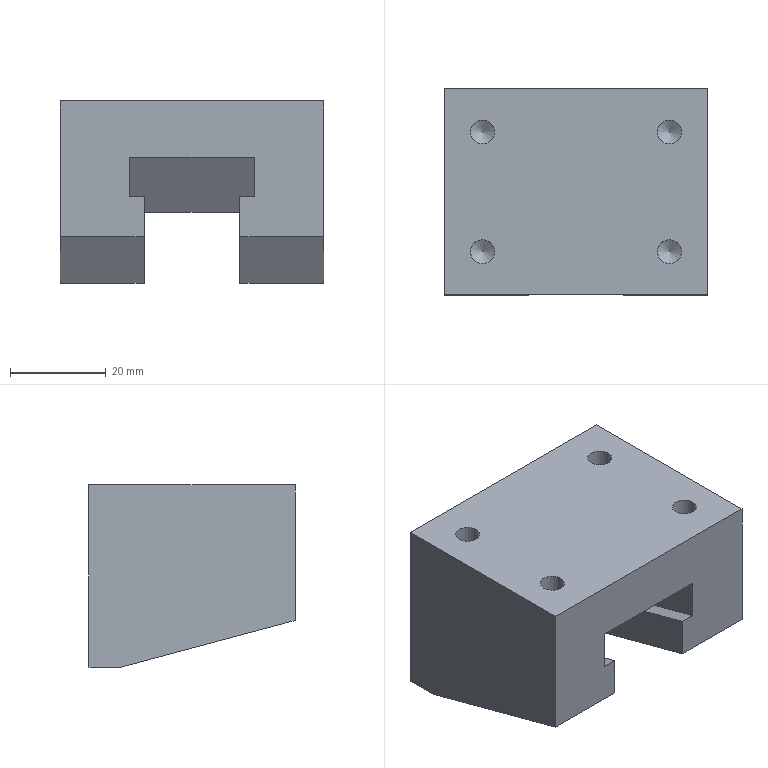Part | STEP file | lll_id478_x_t | 1 solid | 24 faces | box 55 x 43 x 38 mm | volume 62976 mm3 | plane 16 | cone 4 | cylinder 4 | commonest cylinder face diameters 5 x4
STEP:
#1=CARTESIAN_POINT('',(-27.5,108.,137.5));
#2=VERTEX_POINT('',#1);
#3=CARTESIAN_POINT('',(-27.5,108.,99.5));
#4=VERTEX_POINT('',#3);
#5=CARTESIAN_POINT('',(-27.5,108.,83.875));
#6=DIRECTION('',(0.,0.,-1.));
#7=VECTOR('',#6,1.);
#8=LINE('',#5,#7);
#9=EDGE_CURVE('',#2,#4,#8,.T.);
#10=ORIENTED_EDGE('',*,*,#9,.T.);
#11=CARTESIAN_POINT('',(-27.5,101.196,99.5));
#12=VERTEX_POINT('',#11);
#13=CARTESIAN_POINT('',(-27.5,140.161,99.5));
#14=DIRECTION('',(0.,-1.,0.));
#15=VECTOR('',#14,1.);
#16=LINE('',#13,#15);
#17=EDGE_CURVE('',#4,#12,#16,.T.);
#18=ORIENTED_EDGE('',*,*,#17,.T.);
#19=CARTESIAN_POINT('',(-27.5,65.,109.199));
#20=VERTEX_POINT('',#19);
#21=CARTESIAN_POINT('',(-27.5,141.457,88.712));
#22=DIRECTION('',(0.,0.9659,-0.2588));
#23=VECTOR('',#22,1.);
#24=LINE('',#21,#23);
#25=EDGE_CURVE('',#20,#12,#24,.T.);
#26=ORIENTED_EDGE('',*,*,#25,.F.);
#27=CARTESIAN_POINT('',(-27.5,65.,137.5));
#28=VERTEX_POINT('',#27);
#29=CARTESIAN_POINT('',(-27.5,65.,30.5));
#30=DIRECTION('',(0.,0.,-1.));
#31=VECTOR('',#30,1.);
#32=LINE('',#29,#31);
#33=EDGE_CURVE('',#28,#20,#32,.T.);
#34=ORIENTED_EDGE('',*,*,#33,.F.);
#35=CARTESIAN_POINT('',(-27.5,0.,137.5));
#36=DIRECTION('',(0.,-1.,0.));
#37=VECTOR('',#36,1.);
#38=LINE('',#35,#37);
#39=EDGE_CURVE('',#2,#28,#38,.T.);
#40=ORIENTED_EDGE('',*,*,#39,.F.);
#41=EDGE_LOOP('',(#10,#18,#26,#34,#40));
#42=FACE_OUTER_BOUND('',#41,.T.);
#43=CARTESIAN_POINT('',(-27.5,140.161,83.875));
#44=DIRECTION('',(-1.,0.,0.));
#45=DIRECTION('',(0.,0.,1.));
#46=AXIS2_PLACEMENT_3D('',#43,#44,#45);
#47=PLANE('',#46);
#48=ADVANCED_FACE('',(#42),#47,.T.);
#49=CARTESIAN_POINT('',(27.5,101.196,99.5));
#50=VERTEX_POINT('',#49);
#51=CARTESIAN_POINT('',(27.5,65.,109.199));
#52=VERTEX_POINT('',#51);
#53=CARTESIAN_POINT('',(27.5,141.457,88.712));
#54=DIRECTION('',(0.,-0.9659,0.2588));
#55=VECTOR('',#54,1.);
#56=LINE('',#53,#55);
#57=EDGE_CURVE('',#50,#52,#56,.T.);
#58=ORIENTED_EDGE('',*,*,#57,.F.);
#59=CARTESIAN_POINT('',(27.5,108.,99.5));
#60=VERTEX_POINT('',#59);
#61=CARTESIAN_POINT('',(27.5,140.161,99.5));
#62=DIRECTION('',(0.,1.,0.));
#63=VECTOR('',#62,1.);
#64=LINE('',#61,#63);
#65=EDGE_CURVE('',#50,#60,#64,.T.);
#66=ORIENTED_EDGE('',*,*,#65,.T.);
#67=CARTESIAN_POINT('',(27.5,108.,137.5));
#68=VERTEX_POINT('',#67);
#69=CARTESIAN_POINT('',(27.5,108.,83.875));
#70=DIRECTION('',(0.,0.,1.));
#71=VECTOR('',#70,1.);
#72=LINE('',#69,#71);
#73=EDGE_CURVE('',#60,#68,#72,.T.);
#74=ORIENTED_EDGE('',*,*,#73,.T.);
#75=CARTESIAN_POINT('',(27.5,65.,137.5));
#76=VERTEX_POINT('',#75);
#77=CARTESIAN_POINT('',(27.5,140.161,137.5));
#78=DIRECTION('',(0.,-1.,0.));
#79=VECTOR('',#78,1.);
#80=LINE('',#77,#79);
#81=EDGE_CURVE('',#68,#76,#80,.T.);
#82=ORIENTED_EDGE('',*,*,#81,.T.);
#83=CARTESIAN_POINT('',(27.5,65.,83.875));
#84=DIRECTION('',(0.,0.,-1.));
#85=VECTOR('',#84,1.);
#86=LINE('',#83,#85);
#87=EDGE_CURVE('',#76,#52,#86,.T.);
#88=ORIENTED_EDGE('',*,*,#87,.T.);
#89=EDGE_LOOP('',(#58,#66,#74,#82,#88));
#90=FACE_OUTER_BOUND('',#89,.T.);
#91=CARTESIAN_POINT('',(27.5,140.161,83.875));
#92=DIRECTION('',(1.,0.,0.));
#93=DIRECTION('',(0.,0.,-1.));
#94=AXIS2_PLACEMENT_3D('',#91,#92,#93);
#95=PLANE('',#94);
#96=ADVANCED_FACE('',(#90),#95,.T.);
#97=ORIENTED_EDGE('',*,*,#73,.F.);
#98=CARTESIAN_POINT('',(10.,108.,99.5));
#99=VERTEX_POINT('',#98);
#100=CARTESIAN_POINT('',(0.,108.,99.5));
#101=DIRECTION('',(-1.,0.,0.));
#102=VECTOR('',#101,1.);
#103=LINE('',#100,#102);
#104=EDGE_CURVE('',#60,#99,#103,.T.);
#105=ORIENTED_EDGE('',*,*,#104,.T.);
#106=CARTESIAN_POINT('',(10.,108.,105.959));
#107=VERTEX_POINT('',#106);
#108=CARTESIAN_POINT('',(10.,108.,30.5));
#109=DIRECTION('',(0.,0.,-1.));
#110=VECTOR('',#109,1.);
#111=LINE('',#108,#110);
#112=EDGE_CURVE('',#107,#99,#111,.T.);
#113=ORIENTED_EDGE('',*,*,#112,.F.);
#114=CARTESIAN_POINT('',(13.,108.,105.959));
#115=VERTEX_POINT('',#114);
#116=CARTESIAN_POINT('',(0.,108.,105.959));
#117=DIRECTION('',(-1.,0.,0.));
#118=VECTOR('',#117,1.);
#119=LINE('',#116,#118);
#120=EDGE_CURVE('',#115,#107,#119,.T.);
#121=ORIENTED_EDGE('',*,*,#120,.F.);
#122=CARTESIAN_POINT('',(13.,108.,114.241));
#123=VERTEX_POINT('',#122);
#124=CARTESIAN_POINT('',(13.,108.,30.5));
#125=DIRECTION('',(0.,0.,-1.));
#126=VECTOR('',#125,1.);
#127=LINE('',#124,#126);
#128=EDGE_CURVE('',#123,#115,#127,.T.);
#129=ORIENTED_EDGE('',*,*,#128,.F.);
#130=CARTESIAN_POINT('',(-13.,108.,114.241));
#131=VERTEX_POINT('',#130);
#132=CARTESIAN_POINT('',(0.,108.,114.241));
#133=DIRECTION('',(-1.,0.,0.));
#134=VECTOR('',#133,1.);
#135=LINE('',#132,#134);
#136=EDGE_CURVE('',#123,#131,#135,.T.);
#137=ORIENTED_EDGE('',*,*,#136,.T.);
#138=CARTESIAN_POINT('',(-13.,108.,105.959));
#139=VERTEX_POINT('',#138);
#140=CARTESIAN_POINT('',(-13.,108.,30.5));
#141=DIRECTION('',(0.,0.,-1.));
#142=VECTOR('',#141,1.);
#143=LINE('',#140,#142);
#144=EDGE_CURVE('',#131,#139,#143,.T.);
#145=ORIENTED_EDGE('',*,*,#144,.T.);
#146=CARTESIAN_POINT('',(-10.,108.,105.959));
#147=VERTEX_POINT('',#146);
#148=CARTESIAN_POINT('',(0.,108.,105.959));
#149=DIRECTION('',(-1.,0.,0.));
#150=VECTOR('',#149,1.);
#151=LINE('',#148,#150);
#152=EDGE_CURVE('',#147,#139,#151,.T.);
#153=ORIENTED_EDGE('',*,*,#152,.F.);
#154=CARTESIAN_POINT('',(-10.,108.,99.5));
#155=VERTEX_POINT('',#154);
#156=CARTESIAN_POINT('',(-10.,108.,30.5));
#157=DIRECTION('',(0.,0.,-1.));
#158=VECTOR('',#157,1.);
#159=LINE('',#156,#158);
#160=EDGE_CURVE('',#147,#155,#159,.T.);
#161=ORIENTED_EDGE('',*,*,#160,.T.);
#162=CARTESIAN_POINT('',(0.,108.,99.5));
#163=DIRECTION('',(-1.,0.,0.));
#164=VECTOR('',#163,1.);
#165=LINE('',#162,#164);
#166=EDGE_CURVE('',#155,#4,#165,.T.);
#167=ORIENTED_EDGE('',*,*,#166,.T.);
#168=ORIENTED_EDGE('',*,*,#9,.F.);
#169=CARTESIAN_POINT('',(0.,108.,137.5));
#170=DIRECTION('',(-1.,0.,0.));
#171=VECTOR('',#170,1.);
#172=LINE('',#169,#171);
#173=EDGE_CURVE('',#68,#2,#172,.T.);
#174=ORIENTED_EDGE('',*,*,#173,.F.);
#175=EDGE_LOOP('',(#97,#105,#113,#121,#129,#137,#145,#153,#161,#167,#168,#174));
#176=FACE_OUTER_BOUND('',#175,.T.);
#177=CARTESIAN_POINT('',(0.,108.,30.5));
#178=DIRECTION('',(0.,1.,0.));
#179=DIRECTION('',(0.,0.,1.));
#180=AXIS2_PLACEMENT_3D('',#177,#178,#179);
#181=PLANE('',#180);
#182=ADVANCED_FACE('',(#176),#181,.T.);
#183=CARTESIAN_POINT('',(-10.,101.196,99.5));
#184=VERTEX_POINT('',#183);
#185=CARTESIAN_POINT('',(0.00001281,101.196,99.5));
#186=DIRECTION('',(-1.,0.,0.));
#187=VECTOR('',#186,1.);
#188=LINE('',#185,#187);
#189=EDGE_CURVE('',#184,#12,#188,.T.);
#190=ORIENTED_EDGE('',*,*,#189,.F.);
#191=CARTESIAN_POINT('',(-10.,65.,109.199));
#192=VERTEX_POINT('',#191);
#193=CARTESIAN_POINT('',(-10.,90.,102.5));
#194=DIRECTION('',(0.,0.9659,-0.2588));
#195=VECTOR('',#194,1.);
#196=LINE('',#193,#195);
#197=EDGE_CURVE('',#192,#184,#196,.T.);
#198=ORIENTED_EDGE('',*,*,#197,.F.);
#199=CARTESIAN_POINT('',(0.,65.,109.199));
#200=DIRECTION('',(-1.,0.,0.));
#201=VECTOR('',#200,1.);
#202=LINE('',#199,#201);
#203=EDGE_CURVE('',#192,#20,#202,.T.);
#204=ORIENTED_EDGE('',*,*,#203,.T.);
#205=ORIENTED_EDGE('',*,*,#25,.T.);
#206=EDGE_LOOP('',(#190,#198,#204,#205));
#207=FACE_OUTER_BOUND('',#206,.T.);
#208=CARTESIAN_POINT('',(0.00001281,90.,102.5));
#209=DIRECTION('',(0.,-0.2588,-0.9659));
#210=DIRECTION('',(0.,0.9659,-0.2588));
#211=AXIS2_PLACEMENT_3D('',#208,#209,#210);
#212=PLANE('',#211);
#213=ADVANCED_FACE('',(#207),#212,.T.);
#214=ORIENTED_EDGE('',*,*,#197,.T.);
#215=CARTESIAN_POINT('',(-10.,64.,99.5));
#216=DIRECTION('',(0.,1.,0.));
#217=VECTOR('',#216,1.);
#218=LINE('',#215,#217);
#219=EDGE_CURVE('',#184,#155,#218,.T.);
#220=ORIENTED_EDGE('',*,*,#219,.T.);
#221=ORIENTED_EDGE('',*,*,#160,.F.);
#222=CARTESIAN_POINT('',(-10.,65.,117.481));
#223=VERTEX_POINT('',#222);
#224=CARTESIAN_POINT('',(-10.,79.071,113.711));
#225=DIRECTION('',(0.,-0.9659,0.2588));
#226=VECTOR('',#225,1.);
#227=LINE('',#224,#226);
#228=EDGE_CURVE('',#147,#223,#227,.T.);
#229=ORIENTED_EDGE('',*,*,#228,.T.);
#230=CARTESIAN_POINT('',(-10.,65.,30.5));
#231=DIRECTION('',(0.,0.,1.));
#232=VECTOR('',#231,1.);
#233=LINE('',#230,#232);
#234=EDGE_CURVE('',#192,#223,#233,.T.);
#235=ORIENTED_EDGE('',*,*,#234,.F.);
#236=EDGE_LOOP('',(#214,#220,#221,#229,#235));
#237=FACE_OUTER_BOUND('',#236,.T.);
#238=CARTESIAN_POINT('',(-10.,64.,109.467));
#239=DIRECTION('',(1.,0.,0.));
#240=DIRECTION('',(0.,0.,-1.));
#241=AXIS2_PLACEMENT_3D('',#238,#239,#240);
#242=PLANE('',#241);
#243=ADVANCED_FACE('',(#237),#242,.T.);
#244=CARTESIAN_POINT('',(10.,101.196,99.5));
#245=VERTEX_POINT('',#244);
#246=CARTESIAN_POINT('',(0.00001281,101.196,99.5));
#247=DIRECTION('',(-1.,0.,0.));
#248=VECTOR('',#247,1.);
#249=LINE('',#246,#248);
#250=EDGE_CURVE('',#50,#245,#249,.T.);
#251=ORIENTED_EDGE('',*,*,#250,.F.);
#252=ORIENTED_EDGE('',*,*,#57,.T.);
#253=CARTESIAN_POINT('',(10.,65.,109.199));
#254=VERTEX_POINT('',#253);
#255=CARTESIAN_POINT('',(0.,65.,109.199));
#256=DIRECTION('',(-1.,0.,0.));
#257=VECTOR('',#256,1.);
#258=LINE('',#255,#257);
#259=EDGE_CURVE('',#52,#254,#258,.T.);
#260=ORIENTED_EDGE('',*,*,#259,.T.);
#261=CARTESIAN_POINT('',(10.,90.,102.5));
#262=DIRECTION('',(0.,0.9659,-0.2588));
#263=VECTOR('',#262,1.);
#264=LINE('',#261,#263);
#265=EDGE_CURVE('',#254,#245,#264,.T.);
#266=ORIENTED_EDGE('',*,*,#265,.T.);
#267=EDGE_LOOP('',(#251,#252,#260,#266));
#268=FACE_OUTER_BOUND('',#267,.T.);
#269=CARTESIAN_POINT('',(0.00001281,90.,102.5));
#270=DIRECTION('',(0.,-0.2588,-0.9659));
#271=DIRECTION('',(0.,0.9659,-0.2588));
#272=AXIS2_PLACEMENT_3D('',#269,#270,#271);
#273=PLANE('',#272);
#274=ADVANCED_FACE('',(#268),#273,.T.);
#275=CARTESIAN_POINT('',(10.,64.,99.5));
#276=DIRECTION('',(0.,1.,0.));
#277=VECTOR('',#276,1.);
#278=LINE('',#275,#277);
#279=EDGE_CURVE('',#245,#99,#278,.T.);
#280=ORIENTED_EDGE('',*,*,#279,.F.);
#281=ORIENTED_EDGE('',*,*,#265,.F.);
#282=CARTESIAN_POINT('',(10.,65.,117.481));
#283=VERTEX_POINT('',#282);
#284=CARTESIAN_POINT('',(10.,65.,30.5));
#285=DIRECTION('',(0.,0.,1.));
#286=VECTOR('',#285,1.);
#287=LINE('',#284,#286);
#288=EDGE_CURVE('',#254,#283,#287,.T.);
#289=ORIENTED_EDGE('',*,*,#288,.T.);
#290=CARTESIAN_POINT('',(10.,79.071,113.711));
#291=DIRECTION('',(0.,-0.9659,0.2588));
#292=VECTOR('',#291,1.);
#293=LINE('',#290,#292);
#294=EDGE_CURVE('',#107,#283,#293,.T.);
#295=ORIENTED_EDGE('',*,*,#294,.F.);
#296=ORIENTED_EDGE('',*,*,#112,.T.);
#297=EDGE_LOOP('',(#280,#281,#289,#295,#296));
#298=FACE_OUTER_BOUND('',#297,.T.);
#299=CARTESIAN_POINT('',(10.,64.,109.467));
#300=DIRECTION('',(1.,0.,0.));
#301=DIRECTION('',(0.,0.,-1.));
#302=AXIS2_PLACEMENT_3D('',#299,#300,#301);
#303=PLANE('',#302);
#304=ADVANCED_FACE('',(#298),#303,.F.);
#305=ORIENTED_EDGE('',*,*,#136,.F.);
#306=CARTESIAN_POINT('',(13.,65.,125.763));
#307=VERTEX_POINT('',#306);
#308=CARTESIAN_POINT('',(13.,81.141,121.438));
#309=DIRECTION('',(0.,-0.9659,0.2588));
#310=VECTOR('',#309,1.);
#311=LINE('',#308,#310);
#312=EDGE_CURVE('',#123,#307,#311,.T.);
#313=ORIENTED_EDGE('',*,*,#312,.T.);
#314=CARTESIAN_POINT('',(-13.,65.,125.763));
#315=VERTEX_POINT('',#314);
#316=CARTESIAN_POINT('',(0.,65.,125.763));
#317=DIRECTION('',(1.,0.,0.));
#318=VECTOR('',#317,1.);
#319=LINE('',#316,#318);
#320=EDGE_CURVE('',#315,#307,#319,.T.);
#321=ORIENTED_EDGE('',*,*,#320,.F.);
#322=CARTESIAN_POINT('',(-13.,81.141,121.438));
#323=DIRECTION('',(0.,-0.9659,0.2588));
#324=VECTOR('',#323,1.);
#325=LINE('',#322,#324);
#326=EDGE_CURVE('',#131,#315,#325,.T.);
#327=ORIENTED_EDGE('',*,*,#326,.F.);
#328=EDGE_LOOP('',(#305,#313,#321,#327));
#329=FACE_OUTER_BOUND('',#328,.T.);
#330=CARTESIAN_POINT('',(0.00001281,81.141,121.438));
#331=DIRECTION('',(0.,-0.2588,-0.9659));
#332=DIRECTION('',(0.,0.9659,-0.2588));
#333=AXIS2_PLACEMENT_3D('',#330,#331,#332);
#334=PLANE('',#333);
#335=ADVANCED_FACE('',(#329),#334,.T.);
#336=CARTESIAN_POINT('',(22.,99.,137.5));
#337=VERTEX_POINT('',#336);
#338=CARTESIAN_POINT('',(19.5,99.,137.5));
#339=DIRECTION('',(0.,0.,-1.));
#340=DIRECTION('',(1.,0.,0.));
#341=AXIS2_PLACEMENT_3D('',#338,#339,#340);
#342=CIRCLE('',#341,2.5);
#343=EDGE_CURVE('',#337,#337,#342,.T.);
#344=ORIENTED_EDGE('',*,*,#343,.T.);
#345=EDGE_LOOP('',(#344));
#346=FACE_BOUND('',#345,.T.);
#347=CARTESIAN_POINT('',(22.,74.,137.5));
#348=VERTEX_POINT('',#347);
#349=CARTESIAN_POINT('',(19.5,74.,137.5));
#350=DIRECTION('',(0.,0.,1.));
#351=DIRECTION('',(1.,0.,0.));
#352=AXIS2_PLACEMENT_3D('',#349,#350,#351);
#353=CIRCLE('',#352,2.5);
#354=EDGE_CURVE('',#348,#348,#353,.T.);
#355=ORIENTED_EDGE('',*,*,#354,.F.);
#356=EDGE_LOOP('',(#355));
#357=FACE_BOUND('',#356,.T.);
#358=CARTESIAN_POINT('',(-22.,99.,137.5));
#359=VERTEX_POINT('',#358);
#360=CARTESIAN_POINT('',(-19.5,99.,137.5));
#361=DIRECTION('',(0.,0.,1.));
#362=DIRECTION('',(-1.,0.,0.));
#363=AXIS2_PLACEMENT_3D('',#360,#361,#362);
#364=CIRCLE('',#363,2.5);
#365=EDGE_CURVE('',#359,#359,#364,.T.);
#366=ORIENTED_EDGE('',*,*,#365,.F.);
#367=EDGE_LOOP('',(#366));
#368=FACE_BOUND('',#367,.T.);
#369=CARTESIAN_POINT('',(-22.,74.,137.5));
#370=VERTEX_POINT('',#369);
#371=CARTESIAN_POINT('',(-19.5,74.,137.5));
#372=DIRECTION('',(0.,0.,-1.));
#373=DIRECTION('',(-1.,0.,0.));
#374=AXIS2_PLACEMENT_3D('',#371,#372,#373);
#375=CIRCLE('',#374,2.5);
#376=EDGE_CURVE('',#370,#370,#375,.T.);
#377=ORIENTED_EDGE('',*,*,#376,.T.);
#378=EDGE_LOOP('',(#377));
#379=FACE_BOUND('',#378,.T.);
#380=CARTESIAN_POINT('',(0.,65.,137.5));
#381=DIRECTION('',(-1.,0.,0.));
#382=VECTOR('',#381,1.);
#383=LINE('',#380,#382);
#384=EDGE_CURVE('',#76,#28,#383,.T.);
#385=ORIENTED_EDGE('',*,*,#384,.F.);
#386=ORIENTED_EDGE('',*,*,#81,.F.);
#387=ORIENTED_EDGE('',*,*,#173,.T.);
#388=ORIENTED_EDGE('',*,*,#39,.T.);
#389=EDGE_LOOP('',(#385,#386,#387,#388));
#390=FACE_BOUND('',#389,.T.);
#391=CARTESIAN_POINT('',(0.,0.,137.5));
#392=DIRECTION('',(0.,0.,1.));
#393=DIRECTION('',(1.,0.,0.));
#394=AXIS2_PLACEMENT_3D('',#391,#392,#393);
#395=PLANE('',#394);
#396=ADVANCED_FACE('',(#346,#357,#368,#379,#390),#395,.T.);
#397=ORIENTED_EDGE('',*,*,#33,.T.);
#398=ORIENTED_EDGE('',*,*,#203,.F.);
#399=ORIENTED_EDGE('',*,*,#234,.T.);
#400=CARTESIAN_POINT('',(-13.,65.,117.481));
#401=VERTEX_POINT('',#400);
#402=CARTESIAN_POINT('',(0.,65.,117.481));
#403=DIRECTION('',(1.,0.,0.));
#404=VECTOR('',#403,1.);
#405=LINE('',#402,#404);
#406=EDGE_CURVE('',#401,#223,#405,.T.);
#407=ORIENTED_EDGE('',*,*,#406,.F.);
#408=CARTESIAN_POINT('',(-13.,65.,30.5));
#409=DIRECTION('',(0.,0.,1.));
#410=VECTOR('',#409,1.);
#411=LINE('',#408,#410);
#412=EDGE_CURVE('',#401,#315,#411,.T.);
#413=ORIENTED_EDGE('',*,*,#412,.T.);
#414=ORIENTED_EDGE('',*,*,#320,.T.);
#415=CARTESIAN_POINT('',(13.,65.,117.481));
#416=VERTEX_POINT('',#415);
#417=CARTESIAN_POINT('',(13.,65.,30.5));
#418=DIRECTION('',(0.,0.,1.));
#419=VECTOR('',#418,1.);
#420=LINE('',#417,#419);
#421=EDGE_CURVE('',#416,#307,#420,.T.);
#422=ORIENTED_EDGE('',*,*,#421,.F.);
#423=CARTESIAN_POINT('',(0.,65.,117.481));
#424=DIRECTION('',(1.,0.,0.));
#425=VECTOR('',#424,1.);
#426=LINE('',#423,#425);
#427=EDGE_CURVE('',#283,#416,#426,.T.);
#428=ORIENTED_EDGE('',*,*,#427,.F.);
#429=ORIENTED_EDGE('',*,*,#288,.F.);
#430=ORIENTED_EDGE('',*,*,#259,.F.);
#431=ORIENTED_EDGE('',*,*,#87,.F.);
#432=ORIENTED_EDGE('',*,*,#384,.T.);
#433=EDGE_LOOP('',(#397,#398,#399,#407,#413,#414,#422,#428,#429,#430,#431,#432));
#434=FACE_OUTER_BOUND('',#433,.T.);
#435=CARTESIAN_POINT('',(0.,65.,30.5));
#436=DIRECTION('',(0.,1.,0.));
#437=DIRECTION('',(0.,0.,1.));
#438=AXIS2_PLACEMENT_3D('',#435,#436,#437);
#439=PLANE('',#438);
#440=ADVANCED_FACE('',(#434),#439,.F.);
#441=CARTESIAN_POINT('',(-13.,79.071,113.711));
#442=DIRECTION('',(0.,-0.9659,0.2588));
#443=VECTOR('',#442,1.);
#444=LINE('',#441,#443);
#445=EDGE_CURVE('',#139,#401,#444,.T.);
#446=ORIENTED_EDGE('',*,*,#445,.F.);
#447=ORIENTED_EDGE('',*,*,#144,.F.);
#448=ORIENTED_EDGE('',*,*,#326,.T.);
#449=ORIENTED_EDGE('',*,*,#412,.F.);
#450=EDGE_LOOP('',(#446,#447,#448,#449));
#451=FACE_OUTER_BOUND('',#450,.T.);
#452=CARTESIAN_POINT('',(-13.,64.,109.467));
#453=DIRECTION('',(1.,0.,0.));
#454=DIRECTION('',(0.,0.,-1.));
#455=AXIS2_PLACEMENT_3D('',#452,#453,#454);
#456=PLANE('',#455);
#457=ADVANCED_FACE('',(#451),#456,.T.);
#458=ORIENTED_EDGE('',*,*,#152,.T.);
#459=ORIENTED_EDGE('',*,*,#445,.T.);
#460=ORIENTED_EDGE('',*,*,#406,.T.);
#461=ORIENTED_EDGE('',*,*,#228,.F.);
#462=EDGE_LOOP('',(#458,#459,#460,#461));
#463=FACE_OUTER_BOUND('',#462,.T.);
#464=CARTESIAN_POINT('',(0.00001281,79.071,113.711));
#465=DIRECTION('',(0.,-0.2588,-0.9659));
#466=DIRECTION('',(0.,0.9659,-0.2588));
#467=AXIS2_PLACEMENT_3D('',#464,#465,#466);
#468=PLANE('',#467);
#469=ADVANCED_FACE('',(#463),#468,.F.);
#470=CARTESIAN_POINT('',(13.,79.071,113.711));
#471=DIRECTION('',(0.,-0.9659,0.2588));
#472=VECTOR('',#471,1.);
#473=LINE('',#470,#472);
#474=EDGE_CURVE('',#115,#416,#473,.T.);
#475=ORIENTED_EDGE('',*,*,#474,.F.);
#476=ORIENTED_EDGE('',*,*,#120,.T.);
#477=ORIENTED_EDGE('',*,*,#294,.T.);
#478=ORIENTED_EDGE('',*,*,#427,.T.);
#479=EDGE_LOOP('',(#475,#476,#477,#478));
#480=FACE_OUTER_BOUND('',#479,.T.);
#481=CARTESIAN_POINT('',(0.00001281,79.071,113.711));
#482=DIRECTION('',(0.,-0.2588,-0.9659));
#483=DIRECTION('',(0.,0.9659,-0.2588));
#484=AXIS2_PLACEMENT_3D('',#481,#482,#483);
#485=PLANE('',#484);
#486=ADVANCED_FACE('',(#480),#485,.F.);
#487=ORIENTED_EDGE('',*,*,#474,.T.);
#488=ORIENTED_EDGE('',*,*,#421,.T.);
#489=ORIENTED_EDGE('',*,*,#312,.F.);
#490=ORIENTED_EDGE('',*,*,#128,.T.);
#491=EDGE_LOOP('',(#487,#488,#489,#490));
#492=FACE_OUTER_BOUND('',#491,.T.);
#493=CARTESIAN_POINT('',(13.,64.,109.467));
#494=DIRECTION('',(1.,0.,0.));
#495=DIRECTION('',(0.,0.,-1.));
#496=AXIS2_PLACEMENT_3D('',#493,#494,#495);
#497=PLANE('',#496);
#498=ADVANCED_FACE('',(#492),#497,.F.);
#499=ORIENTED_EDGE('',*,*,#65,.F.);
#500=ORIENTED_EDGE('',*,*,#250,.T.);
#501=ORIENTED_EDGE('',*,*,#279,.T.);
#502=ORIENTED_EDGE('',*,*,#104,.F.);
#503=EDGE_LOOP('',(#499,#500,#501,#502));
#504=FACE_OUTER_BOUND('',#503,.T.);
#505=CARTESIAN_POINT('',(0.,0.,99.5));
#506=DIRECTION('',(0.,0.,-1.));
#507=DIRECTION('',(-1.,0.,0.));
#508=AXIS2_PLACEMENT_3D('',#505,#506,#507);
#509=PLANE('',#508);
#510=ADVANCED_FACE('',(#504),#509,.T.);
#511=ORIENTED_EDGE('',*,*,#17,.F.);
#512=ORIENTED_EDGE('',*,*,#166,.F.);
#513=ORIENTED_EDGE('',*,*,#219,.F.);
#514=ORIENTED_EDGE('',*,*,#189,.T.);
#515=EDGE_LOOP('',(#511,#512,#513,#514));
#516=FACE_OUTER_BOUND('',#515,.T.);
#517=CARTESIAN_POINT('',(0.,0.,99.5));
#518=DIRECTION('',(0.,0.,-1.));
#519=DIRECTION('',(-1.,0.,0.));
#520=AXIS2_PLACEMENT_3D('',#517,#518,#519);
#521=PLANE('',#520);
#522=ADVANCED_FACE('',(#516),#521,.T.);
#523=CARTESIAN_POINT('',(-22.,74.,125.5));
#524=VERTEX_POINT('',#523);
#525=CARTESIAN_POINT('',(-19.5,74.,125.5));
#526=DIRECTION('',(0.,0.,-1.));
#527=DIRECTION('',(-1.,0.,0.));
#528=AXIS2_PLACEMENT_3D('',#525,#526,#527);
#529=CIRCLE('',#528,2.5);
#530=EDGE_CURVE('',#524,#524,#529,.T.);
#531=ORIENTED_EDGE('',*,*,#530,.F.);
#532=EDGE_LOOP('',(#531));
#533=FACE_BOUND('',#532,.T.);
#534=CARTESIAN_POINT('',(-19.5,74.,123.998));
#535=VERTEX_POINT('',#534);
#536=VERTEX_LOOP('',#535);
#537=FACE_BOUND('',#536,.T.);
#538=CARTESIAN_POINT('',(-19.5,74.,125.5));
#539=DIRECTION('',(0.,0.,1.));
#540=DIRECTION('',(1.,0.,0.));
#541=AXIS2_PLACEMENT_3D('',#538,#539,#540);
#542=CONICAL_SURFACE('',#541,2.5,59.);
#543=ADVANCED_FACE('',(#533,#537),#542,.F.);
#544=ORIENTED_EDGE('',*,*,#530,.T.);
#545=EDGE_LOOP('',(#544));
#546=FACE_BOUND('',#545,.T.);
#547=ORIENTED_EDGE('',*,*,#376,.F.);
#548=EDGE_LOOP('',(#547));
#549=FACE_BOUND('',#548,.T.);
#550=CARTESIAN_POINT('',(-19.5,74.,137.5));
#551=DIRECTION('',(0.,0.,-1.));
#552=DIRECTION('',(-1.,0.,0.));
#553=AXIS2_PLACEMENT_3D('',#550,#551,#552);
#554=CYLINDRICAL_SURFACE('',#553,2.5);
#555=ADVANCED_FACE('',(#546,#549),#554,.F.);
#556=CARTESIAN_POINT('',(-22.,99.,125.5));
#557=VERTEX_POINT('',#556);
#558=CARTESIAN_POINT('',(-19.5,99.,125.5));
#559=DIRECTION('',(0.,0.,1.));
#560=DIRECTION('',(-1.,0.,0.));
#561=AXIS2_PLACEMENT_3D('',#558,#559,#560);
#562=CIRCLE('',#561,2.5);
#563=EDGE_CURVE('',#557,#557,#562,.T.);
#564=ORIENTED_EDGE('',*,*,#563,.T.);
#565=EDGE_LOOP('',(#564));
#566=FACE_BOUND('',#565,.T.);
#567=CARTESIAN_POINT('',(-19.5,99.,123.998));
#568=VERTEX_POINT('',#567);
#569=VERTEX_LOOP('',#568);
#570=FACE_BOUND('',#569,.T.);
#571=CARTESIAN_POINT('',(-19.5,99.,125.5));
#572=DIRECTION('',(0.,0.,1.));
#573=DIRECTION('',(1.,0.,0.));
#574=AXIS2_PLACEMENT_3D('',#571,#572,#573);
#575=CONICAL_SURFACE('',#574,2.5,59.);
#576=ADVANCED_FACE('',(#566,#570),#575,.F.);
#577=ORIENTED_EDGE('',*,*,#563,.F.);
#578=EDGE_LOOP('',(#577));
#579=FACE_BOUND('',#578,.T.);
#580=ORIENTED_EDGE('',*,*,#365,.T.);
#581=EDGE_LOOP('',(#580));
#582=FACE_BOUND('',#581,.T.);
#583=CARTESIAN_POINT('',(-19.5,99.,137.5));
#584=DIRECTION('',(0.,0.,-1.));
#585=DIRECTION('',(-1.,0.,0.));
#586=AXIS2_PLACEMENT_3D('',#583,#584,#585);
#587=CYLINDRICAL_SURFACE('',#586,2.5);
#588=ADVANCED_FACE('',(#579,#582),#587,.F.);
#589=CARTESIAN_POINT('',(22.,74.,125.5));
#590=VERTEX_POINT('',#589);
#591=CARTESIAN_POINT('',(19.5,74.,125.5));
#592=DIRECTION('',(0.,0.,1.));
#593=DIRECTION('',(1.,0.,0.));
#594=AXIS2_PLACEMENT_3D('',#591,#592,#593);
#595=CIRCLE('',#594,2.5);
#596=EDGE_CURVE('',#590,#590,#595,.T.);
#597=ORIENTED_EDGE('',*,*,#596,.T.);
#598=EDGE_LOOP('',(#597));
#599=FACE_BOUND('',#598,.T.);
#600=CARTESIAN_POINT('',(19.5,74.,123.998));
#601=VERTEX_POINT('',#600);
#602=VERTEX_LOOP('',#601);
#603=FACE_BOUND('',#602,.T.);
#604=CARTESIAN_POINT('',(19.5,74.,125.5));
#605=DIRECTION('',(0.,0.,1.));
#606=DIRECTION('',(-1.,0.,0.));
#607=AXIS2_PLACEMENT_3D('',#604,#605,#606);
#608=CONICAL_SURFACE('',#607,2.5,59.);
#609=ADVANCED_FACE('',(#599,#603),#608,.F.);
#610=ORIENTED_EDGE('',*,*,#596,.F.);
#611=EDGE_LOOP('',(#610));
#612=FACE_BOUND('',#611,.T.);
#613=ORIENTED_EDGE('',*,*,#354,.T.);
#614=EDGE_LOOP('',(#613));
#615=FACE_BOUND('',#614,.T.);
#616=CARTESIAN_POINT('',(19.5,74.,137.5));
#617=DIRECTION('',(0.,0.,-1.));
#618=DIRECTION('',(1.,0.,0.));
#619=AXIS2_PLACEMENT_3D('',#616,#617,#618);
#620=CYLINDRICAL_SURFACE('',#619,2.5);
#621=ADVANCED_FACE('',(#612,#615),#620,.F.);
#622=CARTESIAN_POINT('',(22.,99.,125.5));
#623=VERTEX_POINT('',#622);
#624=CARTESIAN_POINT('',(19.5,99.,125.5));
#625=DIRECTION('',(0.,0.,-1.));
#626=DIRECTION('',(1.,0.,0.));
#627=AXIS2_PLACEMENT_3D('',#624,#625,#626);
#628=CIRCLE('',#627,2.5);
#629=EDGE_CURVE('',#623,#623,#628,.T.);
#630=ORIENTED_EDGE('',*,*,#629,.F.);
#631=EDGE_LOOP('',(#630));
#632=FACE_BOUND('',#631,.T.);
#633=CARTESIAN_POINT('',(19.5,99.,123.998));
#634=VERTEX_POINT('',#633);
#635=VERTEX_LOOP('',#634);
#636=FACE_BOUND('',#635,.T.);
#637=CARTESIAN_POINT('',(19.5,99.,125.5));
#638=DIRECTION('',(0.,0.,1.));
#639=DIRECTION('',(-1.,0.,0.));
#640=AXIS2_PLACEMENT_3D('',#637,#638,#639);
#641=CONICAL_SURFACE('',#640,2.5,59.);
#642=ADVANCED_FACE('',(#632,#636),#641,.F.);
#643=ORIENTED_EDGE('',*,*,#629,.T.);
#644=EDGE_LOOP('',(#643));
#645=FACE_BOUND('',#644,.T.);
#646=ORIENTED_EDGE('',*,*,#343,.F.);
#647=EDGE_LOOP('',(#646));
#648=FACE_BOUND('',#647,.T.);
#649=CARTESIAN_POINT('',(19.5,99.,137.5));
#650=DIRECTION('',(0.,0.,-1.));
#651=DIRECTION('',(1.,0.,0.));
#652=AXIS2_PLACEMENT_3D('',#649,#650,#651);
#653=CYLINDRICAL_SURFACE('',#652,2.5);
#654=ADVANCED_FACE('',(#645,#648),#653,.F.);
#655=CLOSED_SHELL('',(#48,#96,#182,#213,#243,#274,#304,#335,#396,#440,#457,#469,#486,#498,#510,#522,#543,#555,#576,#588,#609,#621,#642,#654));
#656=MANIFOLD_SOLID_BREP('',#655);
#657=(LENGTH_UNIT()NAMED_UNIT(*)SI_UNIT(.MILLI.,.METRE.));
#658=UNCERTAINTY_MEASURE_WITH_UNIT(LENGTH_MEASURE(0.00002),#657,'','');
#659=(NAMED_UNIT(*)PLANE_ANGLE_UNIT()SI_UNIT($,.RADIAN.));
#660=PLANE_ANGLE_MEASURE_WITH_UNIT(PLANE_ANGLE_MEASURE(0.01745),#659);
#661=DIMENSIONAL_EXPONENTS(0.,0.,0.,0.,0.,0.,0.);
#662=(CONVERSION_BASED_UNIT('DEGREE',#660)NAMED_UNIT(#661)PLANE_ANGLE_UNIT());
#663=(NAMED_UNIT(*)SI_UNIT($,.STERADIAN.)SOLID_ANGLE_UNIT());
#664=(GEOMETRIC_REPRESENTATION_CONTEXT(3)GLOBAL_UNCERTAINTY_ASSIGNED_CONTEXT((#658))GLOBAL_UNIT_ASSIGNED_CONTEXT((#657,#662,#663))REPRESENTATION_CONTEXT('',''));
#665=ADVANCED_BREP_SHAPE_REPRESENTATION('',(#656),#664);